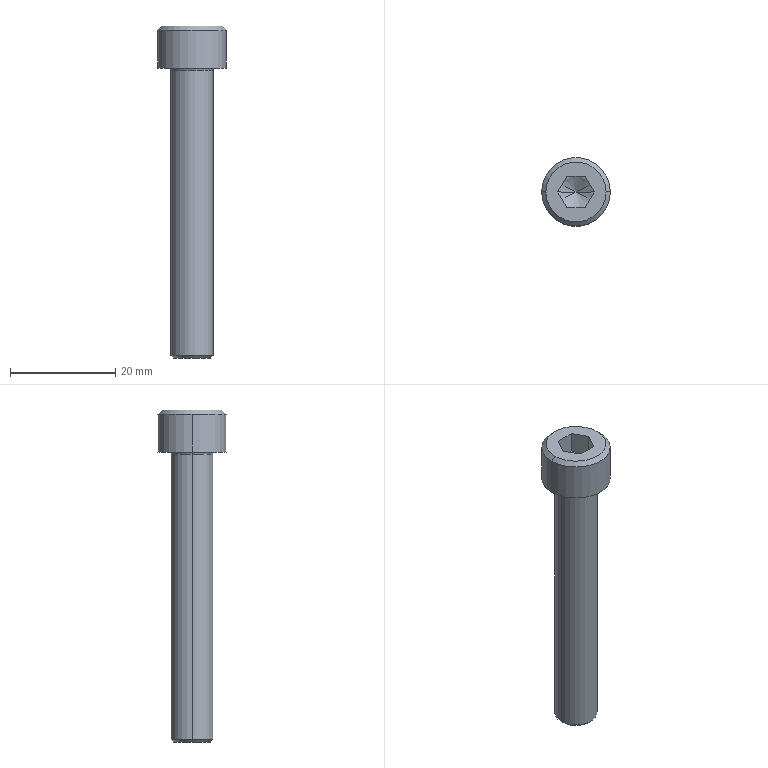Part | Creo | 1 solid | 23 faces | box 13 x 13 x 63 mm | volume 3663 mm3 | plane 9 | cone 6 | cylinder 4 | torus 4 | commonest cylinder face diameters 8 x2 13 x2
STEP:
#1=CARTESIAN_POINT('',(-87.277,359.92,-16.));
#2=VERTEX_POINT('',#1);
#3=CARTESIAN_POINT('',(-89.01,362.92,-16.));
#4=VERTEX_POINT('',#3);
#5=CARTESIAN_POINT('',(-87.277,359.92,-16.));
#6=CARTESIAN_POINT('',(-87.333,360.016,-16.032));
#7=CARTESIAN_POINT('',(-87.442,360.204,-16.09));
#8=CARTESIAN_POINT('',(-87.599,360.476,-16.16));
#9=CARTESIAN_POINT('',(-87.753,360.744,-16.213));
#10=CARTESIAN_POINT('',(-87.908,361.012,-16.25));
#11=CARTESIAN_POINT('',(-88.065,361.284,-16.269));
#12=CARTESIAN_POINT('',(-88.222,361.556,-16.269));
#13=CARTESIAN_POINT('',(-88.379,361.828,-16.25));
#14=CARTESIAN_POINT('',(-88.534,362.096,-16.213));
#15=CARTESIAN_POINT('',(-88.688,362.364,-16.16));
#16=CARTESIAN_POINT('',(-88.846,362.636,-16.09));
#17=CARTESIAN_POINT('',(-88.954,362.824,-16.032));
#18=CARTESIAN_POINT('',(-89.01,362.92,-16.));
#19=B_SPLINE_CURVE_WITH_KNOTS('',3,(#5,#6,#7,#8,#9,#10,#11,#12,#13,#14,#15,#16,#17,#18),.UNSPECIFIED.,.F.,.F.,(4,1,1,1,1,1,1,1,1,1,1,4),(0.,0.09091,0.1818,0.2727,0.3636,0.4545,0.5455,0.6364,0.7273,0.8182,0.9091,1.),.UNSPECIFIED.);
#20=EDGE_CURVE('',#2,#4,#19,.T.);
#21=ORIENTED_EDGE('',*,*,#20,.F.);
#22=CARTESIAN_POINT('',(-90.742,359.92,-18.));
#23=VERTEX_POINT('',#22);
#24=CARTESIAN_POINT('',(-90.742,359.92,-18.));
#25=DIRECTION('',(0.866,0.,0.5));
#26=VECTOR('',#25,4.);
#27=LINE('',#24,#26);
#28=EDGE_CURVE('',#23,#2,#27,.T.);
#29=ORIENTED_EDGE('',*,*,#28,.F.);
#30=CARTESIAN_POINT('',(-94.206,359.92,-16.));
#31=VERTEX_POINT('',#30);
#32=CARTESIAN_POINT('',(-90.742,359.92,-18.));
#33=DIRECTION('',(-0.866,0.,0.5));
#34=VECTOR('',#33,4.);
#35=LINE('',#32,#34);
#36=EDGE_CURVE('',#23,#31,#35,.T.);
#37=ORIENTED_EDGE('',*,*,#36,.T.);
#38=CARTESIAN_POINT('',(-92.474,362.92,-16.));
#39=VERTEX_POINT('',#38);
#40=CARTESIAN_POINT('',(-92.474,362.92,-16.));
#41=CARTESIAN_POINT('',(-92.529,362.824,-16.032));
#42=CARTESIAN_POINT('',(-92.638,362.636,-16.09));
#43=CARTESIAN_POINT('',(-92.795,362.364,-16.16));
#44=CARTESIAN_POINT('',(-92.949,362.096,-16.213));
#45=CARTESIAN_POINT('',(-93.104,361.828,-16.25));
#46=CARTESIAN_POINT('',(-93.261,361.556,-16.269));
#47=CARTESIAN_POINT('',(-93.418,361.284,-16.269));
#48=CARTESIAN_POINT('',(-93.575,361.012,-16.25));
#49=CARTESIAN_POINT('',(-93.73,360.744,-16.213));
#50=CARTESIAN_POINT('',(-93.885,360.476,-16.16));
#51=CARTESIAN_POINT('',(-94.042,360.204,-16.09));
#52=CARTESIAN_POINT('',(-94.15,360.016,-16.032));
#53=CARTESIAN_POINT('',(-94.206,359.92,-16.));
#54=B_SPLINE_CURVE_WITH_KNOTS('',3,(#40,#41,#42,#43,#44,#45,#46,#47,#48,#49,#50,#51,#52,#53),.UNSPECIFIED.,.F.,.F.,(4,1,1,1,1,1,1,1,1,1,1,4),(0.,0.09091,0.1818,0.2727,0.3636,0.4545,0.5455,0.6364,0.7273,0.8182,0.9091,1.),.UNSPECIFIED.);
#55=EDGE_CURVE('',#39,#31,#54,.T.);
#56=ORIENTED_EDGE('',*,*,#55,.F.);
#57=CARTESIAN_POINT('',(-89.01,362.92,-16.));
#58=CARTESIAN_POINT('',(-89.12,362.92,-16.032));
#59=CARTESIAN_POINT('',(-89.337,362.92,-16.09));
#60=CARTESIAN_POINT('',(-89.651,362.92,-16.16));
#61=CARTESIAN_POINT('',(-89.959,362.92,-16.213));
#62=CARTESIAN_POINT('',(-90.269,362.92,-16.25));
#63=CARTESIAN_POINT('',(-90.584,362.92,-16.269));
#64=CARTESIAN_POINT('',(-90.899,362.92,-16.269));
#65=CARTESIAN_POINT('',(-91.214,362.92,-16.25));
#66=CARTESIAN_POINT('',(-91.524,362.92,-16.213));
#67=CARTESIAN_POINT('',(-91.832,362.92,-16.16));
#68=CARTESIAN_POINT('',(-92.146,362.92,-16.09));
#69=CARTESIAN_POINT('',(-92.363,362.92,-16.032));
#70=CARTESIAN_POINT('',(-92.474,362.92,-16.));
#71=B_SPLINE_CURVE_WITH_KNOTS('',3,(#57,#58,#59,#60,#61,#62,#63,#64,#65,#66,#67,#68,#69,#70),.UNSPECIFIED.,.F.,.F.,(4,1,1,1,1,1,1,1,1,1,1,4),(0.,0.09091,0.1818,0.2727,0.3636,0.4545,0.5455,0.6364,0.7273,0.8182,0.9091,1.),.UNSPECIFIED.);
#72=EDGE_CURVE('',#4,#39,#71,.T.);
#73=ORIENTED_EDGE('',*,*,#72,.F.);
#74=EDGE_LOOP('',(#21,#29,#37,#56,#73));
#75=FACE_OUTER_BOUND('',#74,.F.);
#76=CARTESIAN_POINT('',(-90.742,359.92,-16.98));
#77=DIRECTION('',(0.,0.,1.));
#78=DIRECTION('',(1.,0.,0.));
#79=AXIS2_PLACEMENT_3D('',#76,#77,#78);
#80=CONICAL_SURFACE('',#79,1.767,60.);
#81=ADVANCED_FACE('',(#75),#80,.F.);
#82=CARTESIAN_POINT('',(-89.01,362.92,-12.));
#83=VERTEX_POINT('',#82);
#84=CARTESIAN_POINT('',(-87.277,359.92,-12.));
#85=VERTEX_POINT('',#84);
#86=CARTESIAN_POINT('',(-89.01,362.92,-12.));
#87=DIRECTION('',(0.5,-0.866,0.));
#88=VECTOR('',#87,3.464);
#89=LINE('',#86,#88);
#90=EDGE_CURVE('',#83,#85,#89,.T.);
#91=ORIENTED_EDGE('',*,*,#90,.T.);
#92=CARTESIAN_POINT('',(-87.277,359.92,-12.));
#93=DIRECTION('',(0.,0.,-1.));
#94=VECTOR('',#93,4.);
#95=LINE('',#92,#94);
#96=EDGE_CURVE('',#85,#2,#95,.T.);
#97=ORIENTED_EDGE('',*,*,#96,.T.);
#98=ORIENTED_EDGE('',*,*,#20,.T.);
#99=CARTESIAN_POINT('',(-89.01,362.92,-12.));
#100=DIRECTION('',(0.,0.,-1.));
#101=VECTOR('',#100,4.);
#102=LINE('',#99,#101);
#103=EDGE_CURVE('',#83,#4,#102,.T.);
#104=ORIENTED_EDGE('',*,*,#103,.F.);
#105=EDGE_LOOP('',(#91,#97,#98,#104));
#106=FACE_OUTER_BOUND('',#105,.F.);
#107=CARTESIAN_POINT('',(-89.01,362.92,-16.));
#108=DIRECTION('',(-0.866,-0.5,0.));
#109=DIRECTION('',(0.5,-0.866,0.));
#110=AXIS2_PLACEMENT_3D('',#107,#108,#109);
#111=PLANE('',#110);
#112=ADVANCED_FACE('',(#106),#111,.T.);
#113=CARTESIAN_POINT('',(-85.042,359.92,-12.));
#114=VERTEX_POINT('',#113);
#115=CARTESIAN_POINT('',(-96.442,359.92,-12.));
#116=VERTEX_POINT('',#115);
#117=CARTESIAN_POINT('',(-90.742,359.92,-12.));
#118=DIRECTION('',(0.,0.,1.));
#119=DIRECTION('',(1.,0.,0.));
#120=AXIS2_PLACEMENT_3D('',#117,#118,#119);
#121=CIRCLE('',#120,5.7);
#122=EDGE_CURVE('',#114,#116,#121,.T.);
#123=ORIENTED_EDGE('',*,*,#122,.F.);
#124=CARTESIAN_POINT('',(-90.742,359.92,-12.));
#125=DIRECTION('',(0.,0.,1.));
#126=DIRECTION('',(-1.,0.,0.));
#127=AXIS2_PLACEMENT_3D('',#124,#125,#126);
#128=CIRCLE('',#127,5.7);
#129=EDGE_CURVE('',#116,#114,#128,.T.);
#130=ORIENTED_EDGE('',*,*,#129,.F.);
#131=EDGE_LOOP('',(#123,#130));
#132=FACE_OUTER_BOUND('',#131,.F.);
#133=CARTESIAN_POINT('',(-89.01,356.92,-12.));
#134=VERTEX_POINT('',#133);
#135=CARTESIAN_POINT('',(-87.277,359.92,-12.));
#136=DIRECTION('',(-0.5,-0.866,0.));
#137=VECTOR('',#136,3.464);
#138=LINE('',#135,#137);
#139=EDGE_CURVE('',#85,#134,#138,.T.);
#140=ORIENTED_EDGE('',*,*,#139,.F.);
#141=ORIENTED_EDGE('',*,*,#90,.F.);
#142=CARTESIAN_POINT('',(-92.474,362.92,-12.));
#143=VERTEX_POINT('',#142);
#144=CARTESIAN_POINT('',(-89.01,362.92,-12.));
#145=DIRECTION('',(-1.,0.,0.));
#146=VECTOR('',#145,3.464);
#147=LINE('',#144,#146);
#148=EDGE_CURVE('',#83,#143,#147,.T.);
#149=ORIENTED_EDGE('',*,*,#148,.T.);
#150=CARTESIAN_POINT('',(-94.206,359.92,-12.));
#151=VERTEX_POINT('',#150);
#152=CARTESIAN_POINT('',(-94.206,359.92,-12.));
#153=DIRECTION('',(0.5,0.866,0.));
#154=VECTOR('',#153,3.464);
#155=LINE('',#152,#154);
#156=EDGE_CURVE('',#151,#143,#155,.T.);
#157=ORIENTED_EDGE('',*,*,#156,.F.);
#158=CARTESIAN_POINT('',(-92.474,356.92,-12.));
#159=VERTEX_POINT('',#158);
#160=CARTESIAN_POINT('',(-92.474,356.92,-12.));
#161=DIRECTION('',(-0.5,0.866,0.));
#162=VECTOR('',#161,3.464);
#163=LINE('',#160,#162);
#164=EDGE_CURVE('',#159,#151,#163,.T.);
#165=ORIENTED_EDGE('',*,*,#164,.F.);
#166=CARTESIAN_POINT('',(-92.474,356.92,-12.));
#167=DIRECTION('',(1.,0.,0.));
#168=VECTOR('',#167,3.464);
#169=LINE('',#166,#168);
#170=EDGE_CURVE('',#159,#134,#169,.T.);
#171=ORIENTED_EDGE('',*,*,#170,.T.);
#172=EDGE_LOOP('',(#140,#141,#149,#157,#165,#171));
#173=FACE_BOUND('',#172,.F.);
#174=CARTESIAN_POINT('',(-90.742,359.92,-12.));
#175=DIRECTION('',(0.,0.,1.));
#176=DIRECTION('',(1.,0.,0.));
#177=AXIS2_PLACEMENT_3D('',#174,#175,#176);
#178=PLANE('',#177);
#179=ADVANCED_FACE('',(#132,#173),#178,.T.);
#180=CARTESIAN_POINT('',(-84.242,359.92,-12.8));
#181=VERTEX_POINT('',#180);
#182=CARTESIAN_POINT('',(-97.242,359.92,-12.8));
#183=VERTEX_POINT('',#182);
#184=CARTESIAN_POINT('',(-90.742,359.92,-12.8));
#185=DIRECTION('',(0.,0.,1.));
#186=DIRECTION('',(1.,0.,0.));
#187=AXIS2_PLACEMENT_3D('',#184,#185,#186);
#188=CIRCLE('',#187,6.5);
#189=EDGE_CURVE('',#181,#183,#188,.T.);
#190=ORIENTED_EDGE('',*,*,#189,.F.);
#191=CARTESIAN_POINT('',(-85.042,359.92,-12.));
#192=DIRECTION('',(0.7071,0.,-0.7071));
#193=VECTOR('',#192,1.131);
#194=LINE('',#191,#193);
#195=EDGE_CURVE('',#114,#181,#194,.T.);
#196=ORIENTED_EDGE('',*,*,#195,.F.);
#197=ORIENTED_EDGE('',*,*,#122,.T.);
#198=CARTESIAN_POINT('',(-96.442,359.92,-12.));
#199=DIRECTION('',(-0.7071,0.,-0.7071));
#200=VECTOR('',#199,1.131);
#201=LINE('',#198,#200);
#202=EDGE_CURVE('',#116,#183,#201,.T.);
#203=ORIENTED_EDGE('',*,*,#202,.T.);
#204=EDGE_LOOP('',(#190,#196,#197,#203));
#205=FACE_OUTER_BOUND('',#204,.F.);
#206=CARTESIAN_POINT('',(-90.742,359.92,-12.4));
#207=DIRECTION('',(0.,0.,-1.));
#208=DIRECTION('',(-1.,0.,0.));
#209=AXIS2_PLACEMENT_3D('',#206,#207,#208);
#210=CONICAL_SURFACE('',#209,6.1,45.);
#211=ADVANCED_FACE('',(#205),#210,.T.);
#212=ORIENTED_EDGE('',*,*,#189,.T.);
#213=CARTESIAN_POINT('',(-97.242,359.92,-20.));
#214=VERTEX_POINT('',#213);
#215=CARTESIAN_POINT('',(-97.242,359.92,-20.));
#216=DIRECTION('',(0.,0.,1.));
#217=VECTOR('',#216,7.2);
#218=LINE('',#215,#217);
#219=EDGE_CURVE('',#214,#183,#218,.T.);
#220=ORIENTED_EDGE('',*,*,#219,.F.);
#221=CARTESIAN_POINT('',(-84.242,359.92,-20.));
#222=VERTEX_POINT('',#221);
#223=CARTESIAN_POINT('',(-90.742,359.92,-20.));
#224=DIRECTION('',(0.,0.,-1.));
#225=DIRECTION('',(-1.,0.,0.));
#226=AXIS2_PLACEMENT_3D('',#223,#224,#225);
#227=CIRCLE('',#226,6.5);
#228=EDGE_CURVE('',#214,#222,#227,.T.);
#229=ORIENTED_EDGE('',*,*,#228,.T.);
#230=CARTESIAN_POINT('',(-84.242,359.92,-20.));
#231=DIRECTION('',(0.,0.,1.));
#232=VECTOR('',#231,7.2);
#233=LINE('',#230,#232);
#234=EDGE_CURVE('',#222,#181,#233,.T.);
#235=ORIENTED_EDGE('',*,*,#234,.T.);
#236=EDGE_LOOP('',(#212,#220,#229,#235));
#237=FACE_OUTER_BOUND('',#236,.F.);
#238=CARTESIAN_POINT('',(-90.742,359.92,-20.));
#239=DIRECTION('',(0.,0.,1.));
#240=DIRECTION('',(1.,0.,0.));
#241=AXIS2_PLACEMENT_3D('',#238,#239,#240);
#242=CYLINDRICAL_SURFACE('',#241,6.5);
#243=ADVANCED_FACE('',(#237),#242,.T.);
#244=CARTESIAN_POINT('',(-90.742,359.92,-12.8));
#245=DIRECTION('',(0.,0.,1.));
#246=DIRECTION('',(-1.,0.,0.));
#247=AXIS2_PLACEMENT_3D('',#244,#245,#246);
#248=CIRCLE('',#247,6.5);
#249=EDGE_CURVE('',#183,#181,#248,.T.);
#250=ORIENTED_EDGE('',*,*,#249,.T.);
#251=ORIENTED_EDGE('',*,*,#234,.F.);
#252=CARTESIAN_POINT('',(-90.742,359.92,-20.));
#253=DIRECTION('',(0.,0.,-1.));
#254=DIRECTION('',(1.,0.,0.));
#255=AXIS2_PLACEMENT_3D('',#252,#253,#254);
#256=CIRCLE('',#255,6.5);
#257=EDGE_CURVE('',#222,#214,#256,.T.);
#258=ORIENTED_EDGE('',*,*,#257,.T.);
#259=ORIENTED_EDGE('',*,*,#219,.T.);
#260=EDGE_LOOP('',(#250,#251,#258,#259));
#261=FACE_OUTER_BOUND('',#260,.F.);
#262=CARTESIAN_POINT('',(-90.742,359.92,-20.));
#263=DIRECTION('',(0.,0.,1.));
#264=DIRECTION('',(1.,0.,0.));
#265=AXIS2_PLACEMENT_3D('',#262,#263,#264);
#266=CYLINDRICAL_SURFACE('',#265,6.5);
#267=ADVANCED_FACE('',(#261),#266,.T.);
#268=ORIENTED_EDGE('',*,*,#249,.F.);
#269=ORIENTED_EDGE('',*,*,#202,.F.);
#270=ORIENTED_EDGE('',*,*,#129,.T.);
#271=ORIENTED_EDGE('',*,*,#195,.T.);
#272=EDGE_LOOP('',(#268,#269,#270,#271));
#273=FACE_OUTER_BOUND('',#272,.F.);
#274=CARTESIAN_POINT('',(-90.742,359.92,-12.4));
#275=DIRECTION('',(0.,0.,-1.));
#276=DIRECTION('',(-1.,0.,0.));
#277=AXIS2_PLACEMENT_3D('',#274,#275,#276);
#278=CONICAL_SURFACE('',#277,6.1,45.);
#279=ADVANCED_FACE('',(#273),#278,.T.);
#280=ORIENTED_EDGE('',*,*,#257,.F.);
#281=ORIENTED_EDGE('',*,*,#228,.F.);
#282=EDGE_LOOP('',(#280,#281));
#283=FACE_OUTER_BOUND('',#282,.F.);
#284=CARTESIAN_POINT('',(-86.342,359.92,-20.));
#285=VERTEX_POINT('',#284);
#286=CARTESIAN_POINT('',(-95.142,359.92,-20.));
#287=VERTEX_POINT('',#286);
#288=CARTESIAN_POINT('',(-90.742,359.92,-20.));
#289=DIRECTION('',(0.,0.,1.));
#290=DIRECTION('',(1.,0.,0.));
#291=AXIS2_PLACEMENT_3D('',#288,#289,#290);
#292=CIRCLE('',#291,4.4);
#293=EDGE_CURVE('',#285,#287,#292,.T.);
#294=ORIENTED_EDGE('',*,*,#293,.F.);
#295=CARTESIAN_POINT('',(-90.742,359.92,-20.));
#296=DIRECTION('',(0.,0.,1.));
#297=DIRECTION('',(-1.,0.,0.));
#298=AXIS2_PLACEMENT_3D('',#295,#296,#297);
#299=CIRCLE('',#298,4.4);
#300=EDGE_CURVE('',#287,#285,#299,.T.);
#301=ORIENTED_EDGE('',*,*,#300,.F.);
#302=EDGE_LOOP('',(#294,#301));
#303=FACE_BOUND('',#302,.F.);
#304=CARTESIAN_POINT('',(-90.742,359.92,-20.));
#305=DIRECTION('',(0.,0.,1.));
#306=DIRECTION('',(1.,0.,0.));
#307=AXIS2_PLACEMENT_3D('',#304,#305,#306);
#308=PLANE('',#307);
#309=ADVANCED_FACE('',(#283,#303),#308,.F.);
#310=ORIENTED_EDGE('',*,*,#293,.T.);
#311=CARTESIAN_POINT('',(-94.859,359.92,-20.117));
#312=VERTEX_POINT('',#311);
#313=CARTESIAN_POINT('',(-95.142,359.92,-20.4));
#314=DIRECTION('',(0.,1.,0.));
#315=DIRECTION('',(0.,0.,1.));
#316=AXIS2_PLACEMENT_3D('',#313,#314,#315);
#317=CIRCLE('',#316,0.4);
#318=EDGE_CURVE('',#287,#312,#317,.T.);
#319=ORIENTED_EDGE('',*,*,#318,.T.);
#320=CARTESIAN_POINT('',(-86.624,359.92,-20.117));
#321=VERTEX_POINT('',#320);
#322=CARTESIAN_POINT('',(-90.742,359.92,-20.117));
#323=DIRECTION('',(0.,0.,1.));
#324=DIRECTION('',(1.,0.,0.));
#325=AXIS2_PLACEMENT_3D('',#322,#323,#324);
#326=CIRCLE('',#325,4.117);
#327=EDGE_CURVE('',#321,#312,#326,.T.);
#328=ORIENTED_EDGE('',*,*,#327,.F.);
#329=CARTESIAN_POINT('',(-86.342,359.92,-20.4));
#330=DIRECTION('',(0.,-1.,0.));
#331=DIRECTION('',(0.,0.,1.));
#332=AXIS2_PLACEMENT_3D('',#329,#330,#331);
#333=CIRCLE('',#332,0.4);
#334=EDGE_CURVE('',#285,#321,#333,.T.);
#335=ORIENTED_EDGE('',*,*,#334,.F.);
#336=EDGE_LOOP('',(#310,#319,#328,#335));
#337=FACE_OUTER_BOUND('',#336,.F.);
#338=CARTESIAN_POINT('',(-90.742,359.92,-20.4));
#339=DIRECTION('',(0.,0.,1.));
#340=DIRECTION('',(1.,0.,0.));
#341=AXIS2_PLACEMENT_3D('',#338,#339,#340);
#342=TOROIDAL_SURFACE('',#341,4.4,0.4);
#343=ADVANCED_FACE('',(#337),#342,.F.);
#344=ORIENTED_EDGE('',*,*,#300,.T.);
#345=ORIENTED_EDGE('',*,*,#334,.T.);
#346=CARTESIAN_POINT('',(-90.742,359.92,-20.117));
#347=DIRECTION('',(0.,0.,1.));
#348=DIRECTION('',(-1.,0.,0.));
#349=AXIS2_PLACEMENT_3D('',#346,#347,#348);
#350=CIRCLE('',#349,4.117);
#351=EDGE_CURVE('',#312,#321,#350,.T.);
#352=ORIENTED_EDGE('',*,*,#351,.F.);
#353=ORIENTED_EDGE('',*,*,#318,.F.);
#354=EDGE_LOOP('',(#344,#345,#352,#353));
#355=FACE_OUTER_BOUND('',#354,.F.);
#356=CARTESIAN_POINT('',(-90.742,359.92,-20.4));
#357=DIRECTION('',(0.,0.,1.));
#358=DIRECTION('',(1.,0.,0.));
#359=AXIS2_PLACEMENT_3D('',#356,#357,#358);
#360=TOROIDAL_SURFACE('',#359,4.4,0.4);
#361=ADVANCED_FACE('',(#355),#360,.F.);
#362=CARTESIAN_POINT('',(-94.742,359.92,-20.4));
#363=VERTEX_POINT('',#362);
#364=CARTESIAN_POINT('',(-86.742,359.92,-20.4));
#365=VERTEX_POINT('',#364);
#366=CARTESIAN_POINT('',(-90.742,359.92,-20.4));
#367=DIRECTION('',(0.,0.,1.));
#368=DIRECTION('',(-1.,0.,0.));
#369=AXIS2_PLACEMENT_3D('',#366,#367,#368);
#370=CIRCLE('',#369,4.);
#371=EDGE_CURVE('',#363,#365,#370,.T.);
#372=ORIENTED_EDGE('',*,*,#371,.F.);
#373=CARTESIAN_POINT('',(-95.142,359.92,-20.4));
#374=DIRECTION('',(0.,1.,0.));
#375=DIRECTION('',(0.7071,0.,0.7071));
#376=AXIS2_PLACEMENT_3D('',#373,#374,#375);
#377=CIRCLE('',#376,0.4);
#378=EDGE_CURVE('',#312,#363,#377,.T.);
#379=ORIENTED_EDGE('',*,*,#378,.F.);
#380=ORIENTED_EDGE('',*,*,#351,.T.);
#381=CARTESIAN_POINT('',(-86.342,359.92,-20.4));
#382=DIRECTION('',(0.,-1.,0.));
#383=DIRECTION('',(-0.7071,0.,0.7071));
#384=AXIS2_PLACEMENT_3D('',#381,#382,#383);
#385=CIRCLE('',#384,0.4);
#386=EDGE_CURVE('',#321,#365,#385,.T.);
#387=ORIENTED_EDGE('',*,*,#386,.T.);
#388=EDGE_LOOP('',(#372,#379,#380,#387));
#389=FACE_OUTER_BOUND('',#388,.F.);
#390=CARTESIAN_POINT('',(-90.742,359.92,-20.4));
#391=DIRECTION('',(0.,0.,1.));
#392=DIRECTION('',(1.,0.,0.));
#393=AXIS2_PLACEMENT_3D('',#390,#391,#392);
#394=TOROIDAL_SURFACE('',#393,4.4,0.4);
#395=ADVANCED_FACE('',(#389),#394,.F.);
#396=CARTESIAN_POINT('',(-86.742,359.92,-74.5));
#397=VERTEX_POINT('',#396);
#398=CARTESIAN_POINT('',(-94.742,359.92,-74.5));
#399=VERTEX_POINT('',#398);
#400=CARTESIAN_POINT('',(-90.742,359.92,-74.5));
#401=DIRECTION('',(0.,0.,-1.));
#402=DIRECTION('',(1.,0.,0.));
#403=AXIS2_PLACEMENT_3D('',#400,#401,#402);
#404=CIRCLE('',#403,4.);
#405=EDGE_CURVE('',#397,#399,#404,.T.);
#406=ORIENTED_EDGE('',*,*,#405,.T.);
#407=CARTESIAN_POINT('',(-94.742,359.92,-74.5));
#408=DIRECTION('',(0.,0.,1.));
#409=VECTOR('',#408,54.1);
#410=LINE('',#407,#409);
#411=EDGE_CURVE('',#399,#363,#410,.T.);
#412=ORIENTED_EDGE('',*,*,#411,.T.);
#413=ORIENTED_EDGE('',*,*,#371,.T.);
#414=CARTESIAN_POINT('',(-86.742,359.92,-74.5));
#415=DIRECTION('',(0.,0.,1.));
#416=VECTOR('',#415,54.1);
#417=LINE('',#414,#416);
#418=EDGE_CURVE('',#397,#365,#417,.T.);
#419=ORIENTED_EDGE('',*,*,#418,.F.);
#420=EDGE_LOOP('',(#406,#412,#413,#419));
#421=FACE_OUTER_BOUND('',#420,.F.);
#422=CARTESIAN_POINT('',(-90.742,359.92,-75.));
#423=DIRECTION('',(0.,0.,1.));
#424=DIRECTION('',(1.,0.,0.));
#425=AXIS2_PLACEMENT_3D('',#422,#423,#424);
#426=CYLINDRICAL_SURFACE('',#425,4.);
#427=ADVANCED_FACE('',(#421),#426,.T.);
#428=CARTESIAN_POINT('',(-87.242,359.92,-75.));
#429=VERTEX_POINT('',#428);
#430=CARTESIAN_POINT('',(-94.242,359.92,-75.));
#431=VERTEX_POINT('',#430);
#432=CARTESIAN_POINT('',(-90.742,359.92,-75.));
#433=DIRECTION('',(0.,0.,-1.));
#434=DIRECTION('',(1.,0.,0.));
#435=AXIS2_PLACEMENT_3D('',#432,#433,#434);
#436=CIRCLE('',#435,3.5);
#437=EDGE_CURVE('',#429,#431,#436,.T.);
#438=ORIENTED_EDGE('',*,*,#437,.T.);
#439=CARTESIAN_POINT('',(-94.242,359.92,-75.));
#440=DIRECTION('',(-0.7071,0.,0.7071));
#441=VECTOR('',#440,0.7071);
#442=LINE('',#439,#441);
#443=EDGE_CURVE('',#431,#399,#442,.T.);
#444=ORIENTED_EDGE('',*,*,#443,.T.);
#445=ORIENTED_EDGE('',*,*,#405,.F.);
#446=CARTESIAN_POINT('',(-87.242,359.92,-75.));
#447=DIRECTION('',(0.7071,0.,0.7071));
#448=VECTOR('',#447,0.7071);
#449=LINE('',#446,#448);
#450=EDGE_CURVE('',#429,#397,#449,.T.);
#451=ORIENTED_EDGE('',*,*,#450,.F.);
#452=EDGE_LOOP('',(#438,#444,#445,#451));
#453=FACE_OUTER_BOUND('',#452,.F.);
#454=CARTESIAN_POINT('',(-90.742,359.92,-74.75));
#455=DIRECTION('',(0.,0.,1.));
#456=DIRECTION('',(1.,0.,0.));
#457=AXIS2_PLACEMENT_3D('',#454,#455,#456);
#458=CONICAL_SURFACE('',#457,3.75,45.);
#459=ADVANCED_FACE('',(#453),#458,.T.);
#460=ORIENTED_EDGE('',*,*,#437,.F.);
#461=CARTESIAN_POINT('',(-90.742,359.92,-75.));
#462=DIRECTION('',(0.,0.,-1.));
#463=DIRECTION('',(-1.,0.,0.));
#464=AXIS2_PLACEMENT_3D('',#461,#462,#463);
#465=CIRCLE('',#464,3.5);
#466=EDGE_CURVE('',#431,#429,#465,.T.);
#467=ORIENTED_EDGE('',*,*,#466,.F.);
#468=EDGE_LOOP('',(#460,#467));
#469=FACE_OUTER_BOUND('',#468,.F.);
#470=CARTESIAN_POINT('',(-90.742,359.92,-75.));
#471=DIRECTION('',(0.,0.,1.));
#472=DIRECTION('',(1.,0.,0.));
#473=AXIS2_PLACEMENT_3D('',#470,#471,#472);
#474=PLANE('',#473);
#475=ADVANCED_FACE('',(#469),#474,.F.);
#476=ORIENTED_EDGE('',*,*,#466,.T.);
#477=ORIENTED_EDGE('',*,*,#450,.T.);
#478=CARTESIAN_POINT('',(-90.742,359.92,-74.5));
#479=DIRECTION('',(0.,0.,-1.));
#480=DIRECTION('',(-1.,0.,0.));
#481=AXIS2_PLACEMENT_3D('',#478,#479,#480);
#482=CIRCLE('',#481,4.);
#483=EDGE_CURVE('',#399,#397,#482,.T.);
#484=ORIENTED_EDGE('',*,*,#483,.F.);
#485=ORIENTED_EDGE('',*,*,#443,.F.);
#486=EDGE_LOOP('',(#476,#477,#484,#485));
#487=FACE_OUTER_BOUND('',#486,.F.);
#488=CARTESIAN_POINT('',(-90.742,359.92,-74.75));
#489=DIRECTION('',(0.,0.,1.));
#490=DIRECTION('',(1.,0.,0.));
#491=AXIS2_PLACEMENT_3D('',#488,#489,#490);
#492=CONICAL_SURFACE('',#491,3.75,45.);
#493=ADVANCED_FACE('',(#487),#492,.T.);
#494=ORIENTED_EDGE('',*,*,#483,.T.);
#495=ORIENTED_EDGE('',*,*,#418,.T.);
#496=CARTESIAN_POINT('',(-90.742,359.92,-20.4));
#497=DIRECTION('',(0.,0.,1.));
#498=DIRECTION('',(1.,0.,0.));
#499=AXIS2_PLACEMENT_3D('',#496,#497,#498);
#500=CIRCLE('',#499,4.);
#501=EDGE_CURVE('',#365,#363,#500,.T.);
#502=ORIENTED_EDGE('',*,*,#501,.T.);
#503=ORIENTED_EDGE('',*,*,#411,.F.);
#504=EDGE_LOOP('',(#494,#495,#502,#503));
#505=FACE_OUTER_BOUND('',#504,.F.);
#506=CARTESIAN_POINT('',(-90.742,359.92,-75.));
#507=DIRECTION('',(0.,0.,1.));
#508=DIRECTION('',(1.,0.,0.));
#509=AXIS2_PLACEMENT_3D('',#506,#507,#508);
#510=CYLINDRICAL_SURFACE('',#509,4.);
#511=ADVANCED_FACE('',(#505),#510,.T.);
#512=ORIENTED_EDGE('',*,*,#501,.F.);
#513=ORIENTED_EDGE('',*,*,#386,.F.);
#514=ORIENTED_EDGE('',*,*,#327,.T.);
#515=ORIENTED_EDGE('',*,*,#378,.T.);
#516=EDGE_LOOP('',(#512,#513,#514,#515));
#517=FACE_OUTER_BOUND('',#516,.F.);
#518=CARTESIAN_POINT('',(-90.742,359.92,-20.4));
#519=DIRECTION('',(0.,0.,1.));
#520=DIRECTION('',(1.,0.,0.));
#521=AXIS2_PLACEMENT_3D('',#518,#519,#520);
#522=TOROIDAL_SURFACE('',#521,4.4,0.4);
#523=ADVANCED_FACE('',(#517),#522,.F.);
#524=ORIENTED_EDGE('',*,*,#139,.T.);
#525=CARTESIAN_POINT('',(-89.01,356.92,-16.));
#526=VERTEX_POINT('',#525);
#527=CARTESIAN_POINT('',(-89.01,356.92,-12.));
#528=DIRECTION('',(0.,0.,-1.));
#529=VECTOR('',#528,4.);
#530=LINE('',#527,#529);
#531=EDGE_CURVE('',#134,#526,#530,.T.);
#532=ORIENTED_EDGE('',*,*,#531,.T.);
#533=CARTESIAN_POINT('',(-89.01,356.92,-16.));
#534=CARTESIAN_POINT('',(-88.954,357.016,-16.032));
#535=CARTESIAN_POINT('',(-88.846,357.204,-16.09));
#536=CARTESIAN_POINT('',(-88.688,357.476,-16.16));
#537=CARTESIAN_POINT('',(-88.534,357.744,-16.213));
#538=CARTESIAN_POINT('',(-88.379,358.012,-16.25));
#539=CARTESIAN_POINT('',(-88.222,358.284,-16.269));
#540=CARTESIAN_POINT('',(-88.065,358.556,-16.269));
#541=CARTESIAN_POINT('',(-87.908,358.828,-16.25));
#542=CARTESIAN_POINT('',(-87.753,359.096,-16.213));
#543=CARTESIAN_POINT('',(-87.599,359.364,-16.16));
#544=CARTESIAN_POINT('',(-87.442,359.636,-16.09));
#545=CARTESIAN_POINT('',(-87.333,359.824,-16.032));
#546=CARTESIAN_POINT('',(-87.277,359.92,-16.));
#547=B_SPLINE_CURVE_WITH_KNOTS('',3,(#533,#534,#535,#536,#537,#538,#539,#540,#541,#542,#543,#544,#545,#546),.UNSPECIFIED.,.F.,.F.,(4,1,1,1,1,1,1,1,1,1,1,4),(0.,0.09091,0.1818,0.2727,0.3636,0.4545,0.5455,0.6364,0.7273,0.8182,0.9091,1.),.UNSPECIFIED.);
#548=EDGE_CURVE('',#526,#2,#547,.T.);
#549=ORIENTED_EDGE('',*,*,#548,.T.);
#550=ORIENTED_EDGE('',*,*,#96,.F.);
#551=EDGE_LOOP('',(#524,#532,#549,#550));
#552=FACE_OUTER_BOUND('',#551,.F.);
#553=CARTESIAN_POINT('',(-87.277,359.92,-16.));
#554=DIRECTION('',(-0.866,0.5,0.));
#555=DIRECTION('',(-0.5,-0.866,0.));
#556=AXIS2_PLACEMENT_3D('',#553,#554,#555);
#557=PLANE('',#556);
#558=ADVANCED_FACE('',(#552),#557,.T.);
#559=ORIENTED_EDGE('',*,*,#170,.F.);
#560=CARTESIAN_POINT('',(-92.474,356.92,-16.));
#561=VERTEX_POINT('',#560);
#562=CARTESIAN_POINT('',(-92.474,356.92,-12.));
#563=DIRECTION('',(0.,0.,-1.));
#564=VECTOR('',#563,4.);
#565=LINE('',#562,#564);
#566=EDGE_CURVE('',#159,#561,#565,.T.);
#567=ORIENTED_EDGE('',*,*,#566,.T.);
#568=CARTESIAN_POINT('',(-92.474,356.92,-16.));
#569=CARTESIAN_POINT('',(-92.363,356.92,-16.032));
#570=CARTESIAN_POINT('',(-92.146,356.92,-16.09));
#571=CARTESIAN_POINT('',(-91.832,356.92,-16.16));
#572=CARTESIAN_POINT('',(-91.524,356.92,-16.213));
#573=CARTESIAN_POINT('',(-91.214,356.92,-16.25));
#574=CARTESIAN_POINT('',(-90.899,356.92,-16.269));
#575=CARTESIAN_POINT('',(-90.584,356.92,-16.269));
#576=CARTESIAN_POINT('',(-90.269,356.92,-16.25));
#577=CARTESIAN_POINT('',(-89.959,356.92,-16.213));
#578=CARTESIAN_POINT('',(-89.651,356.92,-16.16));
#579=CARTESIAN_POINT('',(-89.337,356.92,-16.09));
#580=CARTESIAN_POINT('',(-89.12,356.92,-16.032));
#581=CARTESIAN_POINT('',(-89.01,356.92,-16.));
#582=B_SPLINE_CURVE_WITH_KNOTS('',3,(#568,#569,#570,#571,#572,#573,#574,#575,#576,#577,#578,#579,#580,#581),.UNSPECIFIED.,.F.,.F.,(4,1,1,1,1,1,1,1,1,1,1,4),(0.,0.09091,0.1818,0.2727,0.3636,0.4545,0.5455,0.6364,0.7273,0.8182,0.9091,1.),.UNSPECIFIED.);
#583=EDGE_CURVE('',#561,#526,#582,.T.);
#584=ORIENTED_EDGE('',*,*,#583,.T.);
#585=ORIENTED_EDGE('',*,*,#531,.F.);
#586=EDGE_LOOP('',(#559,#567,#584,#585));
#587=FACE_OUTER_BOUND('',#586,.F.);
#588=CARTESIAN_POINT('',(-89.01,356.92,-16.));
#589=DIRECTION('',(0.,1.,0.));
#590=DIRECTION('',(0.,0.,1.));
#591=AXIS2_PLACEMENT_3D('',#588,#589,#590);
#592=PLANE('',#591);
#593=ADVANCED_FACE('',(#587),#592,.T.);
#594=ORIENTED_EDGE('',*,*,#164,.T.);
#595=CARTESIAN_POINT('',(-94.206,359.92,-12.));
#596=DIRECTION('',(0.,0.,-1.));
#597=VECTOR('',#596,4.);
#598=LINE('',#595,#597);
#599=EDGE_CURVE('',#151,#31,#598,.T.);
#600=ORIENTED_EDGE('',*,*,#599,.T.);
#601=CARTESIAN_POINT('',(-94.206,359.92,-16.));
#602=CARTESIAN_POINT('',(-94.15,359.824,-16.032));
#603=CARTESIAN_POINT('',(-94.042,359.636,-16.09));
#604=CARTESIAN_POINT('',(-93.885,359.364,-16.16));
#605=CARTESIAN_POINT('',(-93.73,359.096,-16.213));
#606=CARTESIAN_POINT('',(-93.575,358.828,-16.25));
#607=CARTESIAN_POINT('',(-93.418,358.556,-16.269));
#608=CARTESIAN_POINT('',(-93.261,358.284,-16.269));
#609=CARTESIAN_POINT('',(-93.104,358.012,-16.25));
#610=CARTESIAN_POINT('',(-92.949,357.744,-16.213));
#611=CARTESIAN_POINT('',(-92.795,357.476,-16.16));
#612=CARTESIAN_POINT('',(-92.638,357.204,-16.09));
#613=CARTESIAN_POINT('',(-92.529,357.016,-16.032));
#614=CARTESIAN_POINT('',(-92.474,356.92,-16.));
#615=B_SPLINE_CURVE_WITH_KNOTS('',3,(#601,#602,#603,#604,#605,#606,#607,#608,#609,#610,#611,#612,#613,#614),.UNSPECIFIED.,.F.,.F.,(4,1,1,1,1,1,1,1,1,1,1,4),(0.,0.09091,0.1818,0.2727,0.3636,0.4545,0.5455,0.6364,0.7273,0.8182,0.9091,1.),.UNSPECIFIED.);
#616=EDGE_CURVE('',#31,#561,#615,.T.);
#617=ORIENTED_EDGE('',*,*,#616,.T.);
#618=ORIENTED_EDGE('',*,*,#566,.F.);
#619=EDGE_LOOP('',(#594,#600,#617,#618));
#620=FACE_OUTER_BOUND('',#619,.F.);
#621=CARTESIAN_POINT('',(-92.474,356.92,-16.));
#622=DIRECTION('',(0.866,0.5,0.));
#623=DIRECTION('',(-0.5,0.866,0.));
#624=AXIS2_PLACEMENT_3D('',#621,#622,#623);
#625=PLANE('',#624);
#626=ADVANCED_FACE('',(#620),#625,.T.);
#627=ORIENTED_EDGE('',*,*,#156,.T.);
#628=CARTESIAN_POINT('',(-92.474,362.92,-12.));
#629=DIRECTION('',(0.,0.,-1.));
#630=VECTOR('',#629,4.);
#631=LINE('',#628,#630);
#632=EDGE_CURVE('',#143,#39,#631,.T.);
#633=ORIENTED_EDGE('',*,*,#632,.T.);
#634=ORIENTED_EDGE('',*,*,#55,.T.);
#635=ORIENTED_EDGE('',*,*,#599,.F.);
#636=EDGE_LOOP('',(#627,#633,#634,#635));
#637=FACE_OUTER_BOUND('',#636,.F.);
#638=CARTESIAN_POINT('',(-94.206,359.92,-16.));
#639=DIRECTION('',(0.866,-0.5,0.));
#640=DIRECTION('',(0.5,0.866,0.));
#641=AXIS2_PLACEMENT_3D('',#638,#639,#640);
#642=PLANE('',#641);
#643=ADVANCED_FACE('',(#637),#642,.T.);
#644=ORIENTED_EDGE('',*,*,#148,.F.);
#645=ORIENTED_EDGE('',*,*,#103,.T.);
#646=ORIENTED_EDGE('',*,*,#72,.T.);
#647=ORIENTED_EDGE('',*,*,#632,.F.);
#648=EDGE_LOOP('',(#644,#645,#646,#647));
#649=FACE_OUTER_BOUND('',#648,.F.);
#650=CARTESIAN_POINT('',(-92.474,362.92,-16.));
#651=DIRECTION('',(0.,-1.,0.));
#652=DIRECTION('',(0.,0.,-1.));
#653=AXIS2_PLACEMENT_3D('',#650,#651,#652);
#654=PLANE('',#653);
#655=ADVANCED_FACE('',(#649),#654,.T.);
#656=ORIENTED_EDGE('',*,*,#616,.F.);
#657=ORIENTED_EDGE('',*,*,#36,.F.);
#658=ORIENTED_EDGE('',*,*,#28,.T.);
#659=ORIENTED_EDGE('',*,*,#548,.F.);
#660=ORIENTED_EDGE('',*,*,#583,.F.);
#661=EDGE_LOOP('',(#656,#657,#658,#659,#660));
#662=FACE_OUTER_BOUND('',#661,.F.);
#663=CARTESIAN_POINT('',(-90.742,359.92,-16.98));
#664=DIRECTION('',(0.,0.,1.));
#665=DIRECTION('',(1.,0.,0.));
#666=AXIS2_PLACEMENT_3D('',#663,#664,#665);
#667=CONICAL_SURFACE('',#666,1.767,60.);
#668=ADVANCED_FACE('',(#662),#667,.F.);
#669=CLOSED_SHELL('',(#81,#112,#179,#211,#243,#267,#279,#309,#343,#361,#395,#427,#459,#475,#493,#511,#523,#558,#593,#626,#643,#655,#668));
#670=MANIFOLD_SOLID_BREP('',#669);
#671=(LENGTH_UNIT()NAMED_UNIT(*)SI_UNIT(.MILLI.,.METRE.));
#672=UNCERTAINTY_MEASURE_WITH_UNIT(LENGTH_MEASURE(0.006563),#671,'','');
#673=(NAMED_UNIT(*)PLANE_ANGLE_UNIT()SI_UNIT($,.RADIAN.));
#674=PLANE_ANGLE_MEASURE_WITH_UNIT(PLANE_ANGLE_MEASURE(0.01745),#673);
#675=(CONVERSION_BASED_UNIT('DEGREE',#674)NAMED_UNIT(*)PLANE_ANGLE_UNIT());
#676=(NAMED_UNIT(*)SI_UNIT($,.STERADIAN.)SOLID_ANGLE_UNIT());
#677=(GEOMETRIC_REPRESENTATION_CONTEXT(3)GLOBAL_UNCERTAINTY_ASSIGNED_CONTEXT((#672))GLOBAL_UNIT_ASSIGNED_CONTEXT((#671,#675,#676))REPRESENTATION_CONTEXT('',''));
#678=ADVANCED_BREP_SHAPE_REPRESENTATION('',(#670),#677);